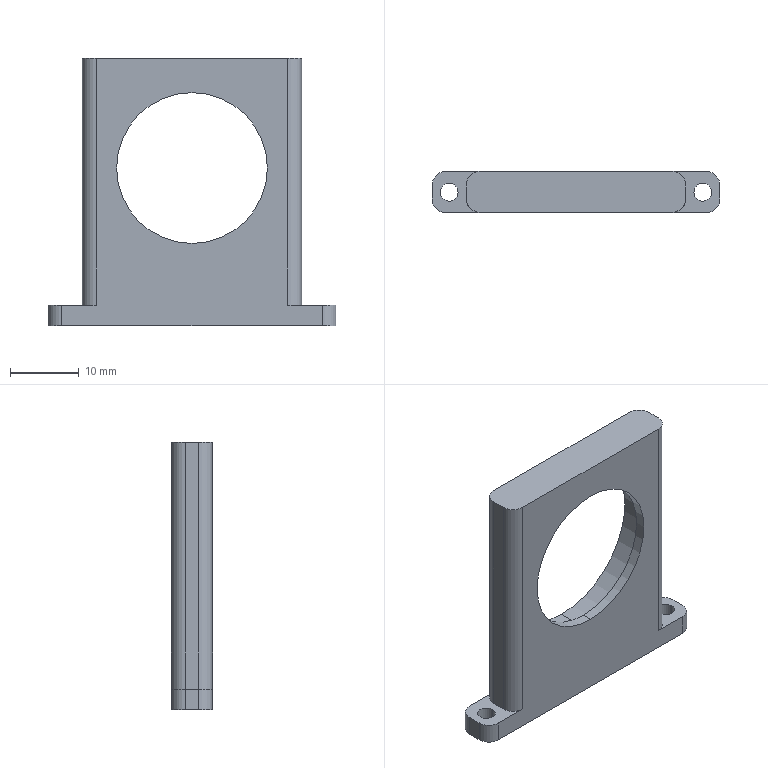Part | NX | 1 solid | 31 faces | box 42 x 6 x 39 mm | volume 4443 mm3 | cylinder 18 | plane 11 | cone 2 | commonest cylinder face diameters 4 x8 2.6 x4 3.3 x2 22 x2 26.2 x2
STEP:
#1=CARTESIAN_POINT('',(1.65,0.,4.009));
#2=VERTEX_POINT('',#1);
#3=CARTESIAN_POINT('',(-1.65,0.,4.009));
#4=VERTEX_POINT('',#3);
#5=CARTESIAN_POINT('',(0.,0.,4.009));
#6=DIRECTION('',(0.,0.,-1.));
#7=DIRECTION('',(-1.,0.,0.));
#8=AXIS2_PLACEMENT_3D('',#5,#6,#7);
#9=CIRCLE('',#8,1.65);
#10=EDGE_CURVE('',#2,#4,#9,.T.);
#11=ORIENTED_EDGE('',*,*,#10,.F.);
#12=CARTESIAN_POINT('',(1.65,0.,-3.));
#13=VERTEX_POINT('',#12);
#14=CARTESIAN_POINT('',(1.65,0.,-3.));
#15=DIRECTION('',(0.,0.,-1.));
#16=VECTOR('',#15,1000.);
#17=LINE('',#14,#16);
#18=EDGE_CURVE('',#2,#13,#17,.T.);
#19=ORIENTED_EDGE('',*,*,#18,.T.);
#20=CARTESIAN_POINT('',(-1.65,0.,-3.));
#21=VERTEX_POINT('',#20);
#22=CARTESIAN_POINT('',(0.,0.,-3.));
#23=DIRECTION('',(0.,0.,-1.));
#24=DIRECTION('',(-1.,0.,0.));
#25=AXIS2_PLACEMENT_3D('',#22,#23,#24);
#26=CIRCLE('',#25,1.65);
#27=EDGE_CURVE('',#13,#21,#26,.T.);
#28=ORIENTED_EDGE('',*,*,#27,.T.);
#29=CARTESIAN_POINT('',(-1.65,0.,-3.));
#30=DIRECTION('',(0.,0.,-1.));
#31=VECTOR('',#30,1000.);
#32=LINE('',#29,#31);
#33=EDGE_CURVE('',#4,#21,#32,.T.);
#34=ORIENTED_EDGE('',*,*,#33,.F.);
#35=EDGE_LOOP('',(#11,#19,#28,#34));
#36=FACE_BOUND('',#35,.T.);
#37=CARTESIAN_POINT('',(0.,0.,-3.));
#38=DIRECTION('',(0.,0.,-1.));
#39=DIRECTION('',(1.,0.,0.));
#40=AXIS2_PLACEMENT_3D('',#37,#38,#39);
#41=CYLINDRICAL_SURFACE('',#40,1.65);
#42=ADVANCED_FACE('',(#36),#41,.F.);
#43=CARTESIAN_POINT('',(0.,0.,5.));
#44=VERTEX_POINT('',#43);
#45=CARTESIAN_POINT('',(-1.65,0.,4.009));
#46=DIRECTION('',(-0.8572,0.,-0.515));
#47=VECTOR('',#46,1000.);
#48=LINE('',#45,#47);
#49=EDGE_CURVE('',#44,#4,#48,.T.);
#50=ORIENTED_EDGE('',*,*,#49,.F.);
#51=CARTESIAN_POINT('',(1.65,0.,4.009));
#52=DIRECTION('',(0.8572,0.,-0.515));
#53=VECTOR('',#52,1000.);
#54=LINE('',#51,#53);
#55=EDGE_CURVE('',#44,#2,#54,.T.);
#56=ORIENTED_EDGE('',*,*,#55,.T.);
#57=ORIENTED_EDGE('',*,*,#10,.T.);
#58=EDGE_LOOP('',(#50,#56,#57));
#59=FACE_BOUND('',#58,.T.);
#60=CARTESIAN_POINT('',(0.,0.,4.009));
#61=DIRECTION('',(0.,0.,-1.));
#62=DIRECTION('',(1.,0.,0.));
#63=AXIS2_PLACEMENT_3D('',#60,#61,#62);
#64=CONICAL_SURFACE('',#63,1.65,1.03);
#65=ADVANCED_FACE('',(#59),#64,.F.);
#66=CARTESIAN_POINT('',(19.8,0.,0.));
#67=VERTEX_POINT('',#66);
#68=CARTESIAN_POINT('',(17.2,0.,0.));
#69=VERTEX_POINT('',#68);
#70=CARTESIAN_POINT('',(18.5,0.,0.));
#71=DIRECTION('',(0.,0.,-1.));
#72=DIRECTION('',(-1.,0.,0.));
#73=AXIS2_PLACEMENT_3D('',#70,#71,#72);
#74=CIRCLE('',#73,1.3);
#75=EDGE_CURVE('',#67,#69,#74,.T.);
#76=ORIENTED_EDGE('',*,*,#75,.F.);
#77=CARTESIAN_POINT('',(19.8,0.,-3.));
#78=VERTEX_POINT('',#77);
#79=CARTESIAN_POINT('',(19.8,0.,36.));
#80=DIRECTION('',(0.,0.,-1.));
#81=VECTOR('',#80,1000.);
#82=LINE('',#79,#81);
#83=EDGE_CURVE('',#67,#78,#82,.T.);
#84=ORIENTED_EDGE('',*,*,#83,.T.);
#85=CARTESIAN_POINT('',(17.2,0.,-3.));
#86=VERTEX_POINT('',#85);
#87=CARTESIAN_POINT('',(18.5,0.,-3.));
#88=DIRECTION('',(0.,0.,-1.));
#89=DIRECTION('',(-1.,0.,0.));
#90=AXIS2_PLACEMENT_3D('',#87,#88,#89);
#91=CIRCLE('',#90,1.3);
#92=EDGE_CURVE('',#78,#86,#91,.T.);
#93=ORIENTED_EDGE('',*,*,#92,.T.);
#94=CARTESIAN_POINT('',(17.2,0.,36.));
#95=DIRECTION('',(0.,0.,-1.));
#96=VECTOR('',#95,1000.);
#97=LINE('',#94,#96);
#98=EDGE_CURVE('',#69,#86,#97,.T.);
#99=ORIENTED_EDGE('',*,*,#98,.F.);
#100=EDGE_LOOP('',(#76,#84,#93,#99));
#101=FACE_BOUND('',#100,.T.);
#102=CARTESIAN_POINT('',(18.5,0.,36.));
#103=DIRECTION('',(0.,0.,-1.));
#104=DIRECTION('',(1.,0.,0.));
#105=AXIS2_PLACEMENT_3D('',#102,#103,#104);
#106=CYLINDRICAL_SURFACE('',#105,1.3);
#107=ADVANCED_FACE('',(#101),#106,.F.);
#108=CARTESIAN_POINT('',(-17.2,0.,0.));
#109=VERTEX_POINT('',#108);
#110=CARTESIAN_POINT('',(-19.8,0.,0.));
#111=VERTEX_POINT('',#110);
#112=CARTESIAN_POINT('',(-18.5,0.,0.));
#113=DIRECTION('',(0.,0.,-1.));
#114=DIRECTION('',(-1.,0.,0.));
#115=AXIS2_PLACEMENT_3D('',#112,#113,#114);
#116=CIRCLE('',#115,1.3);
#117=EDGE_CURVE('',#109,#111,#116,.T.);
#118=ORIENTED_EDGE('',*,*,#117,.F.);
#119=CARTESIAN_POINT('',(-17.2,0.,-3.));
#120=VERTEX_POINT('',#119);
#121=CARTESIAN_POINT('',(-17.2,0.,36.));
#122=DIRECTION('',(0.,0.,-1.));
#123=VECTOR('',#122,1000.);
#124=LINE('',#121,#123);
#125=EDGE_CURVE('',#109,#120,#124,.T.);
#126=ORIENTED_EDGE('',*,*,#125,.T.);
#127=CARTESIAN_POINT('',(-19.8,0.,-3.));
#128=VERTEX_POINT('',#127);
#129=CARTESIAN_POINT('',(-18.5,0.,-3.));
#130=DIRECTION('',(0.,0.,-1.));
#131=DIRECTION('',(-1.,0.,0.));
#132=AXIS2_PLACEMENT_3D('',#129,#130,#131);
#133=CIRCLE('',#132,1.3);
#134=EDGE_CURVE('',#120,#128,#133,.T.);
#135=ORIENTED_EDGE('',*,*,#134,.T.);
#136=CARTESIAN_POINT('',(-19.8,0.,36.));
#137=DIRECTION('',(0.,0.,-1.));
#138=VECTOR('',#137,1000.);
#139=LINE('',#136,#138);
#140=EDGE_CURVE('',#111,#128,#139,.T.);
#141=ORIENTED_EDGE('',*,*,#140,.F.);
#142=EDGE_LOOP('',(#118,#126,#135,#141));
#143=FACE_BOUND('',#142,.T.);
#144=CARTESIAN_POINT('',(-18.5,0.,36.));
#145=DIRECTION('',(0.,0.,-1.));
#146=DIRECTION('',(1.,0.,0.));
#147=AXIS2_PLACEMENT_3D('',#144,#145,#146);
#148=CYLINDRICAL_SURFACE('',#147,1.3);
#149=ADVANCED_FACE('',(#143),#148,.F.);
#150=CARTESIAN_POINT('',(0.,-1.5,6.9));
#151=VERTEX_POINT('',#150);
#152=CARTESIAN_POINT('',(0.,-1.5,33.1));
#153=VERTEX_POINT('',#152);
#154=CARTESIAN_POINT('',(0.,-1.5,20.));
#155=DIRECTION('',(0.,1.,0.));
#156=DIRECTION('',(0.,0.,1.));
#157=AXIS2_PLACEMENT_3D('',#154,#155,#156);
#158=CIRCLE('',#157,13.1);
#159=EDGE_CURVE('',#151,#153,#158,.T.);
#160=ORIENTED_EDGE('',*,*,#159,.F.);
#161=CARTESIAN_POINT('',(0.,3.,6.9));
#162=VERTEX_POINT('',#161);
#163=CARTESIAN_POINT('',(0.,-1.5,6.9));
#164=DIRECTION('',(0.,1.,0.));
#165=VECTOR('',#164,1000.);
#166=LINE('',#163,#165);
#167=EDGE_CURVE('',#151,#162,#166,.T.);
#168=ORIENTED_EDGE('',*,*,#167,.T.);
#169=CARTESIAN_POINT('',(0.,3.,33.1));
#170=VERTEX_POINT('',#169);
#171=CARTESIAN_POINT('',(0.,3.,20.));
#172=DIRECTION('',(0.,1.,0.));
#173=DIRECTION('',(0.,0.,1.));
#174=AXIS2_PLACEMENT_3D('',#171,#172,#173);
#175=CIRCLE('',#174,13.1);
#176=EDGE_CURVE('',#162,#170,#175,.T.);
#177=ORIENTED_EDGE('',*,*,#176,.T.);
#178=CARTESIAN_POINT('',(0.,-1.5,33.1));
#179=DIRECTION('',(0.,1.,0.));
#180=VECTOR('',#179,1000.);
#181=LINE('',#178,#180);
#182=EDGE_CURVE('',#153,#170,#181,.T.);
#183=ORIENTED_EDGE('',*,*,#182,.F.);
#184=EDGE_LOOP('',(#160,#168,#177,#183));
#185=FACE_BOUND('',#184,.T.);
#186=CARTESIAN_POINT('',(0.,-1.5,20.));
#187=DIRECTION('',(0.,1.,0.));
#188=DIRECTION('',(0.,0.,-1.));
#189=AXIS2_PLACEMENT_3D('',#186,#187,#188);
#190=CYLINDRICAL_SURFACE('',#189,13.1);
#191=ADVANCED_FACE('',(#185),#190,.F.);
#192=CARTESIAN_POINT('',(0.,-1.5,31.));
#193=VERTEX_POINT('',#192);
#194=CARTESIAN_POINT('',(0.,-1.5,9.));
#195=VERTEX_POINT('',#194);
#196=CARTESIAN_POINT('',(0.,-1.5,20.));
#197=DIRECTION('',(0.,-1.,0.));
#198=DIRECTION('',(0.,0.,1.));
#199=AXIS2_PLACEMENT_3D('',#196,#197,#198);
#200=CIRCLE('',#199,11.);
#201=EDGE_CURVE('',#193,#195,#200,.T.);
#202=ORIENTED_EDGE('',*,*,#201,.F.);
#203=CARTESIAN_POINT('',(0.,-3.,31.));
#204=VERTEX_POINT('',#203);
#205=CARTESIAN_POINT('',(0.,3.,31.));
#206=DIRECTION('',(0.,-1.,0.));
#207=VECTOR('',#206,1000.);
#208=LINE('',#205,#207);
#209=EDGE_CURVE('',#193,#204,#208,.T.);
#210=ORIENTED_EDGE('',*,*,#209,.T.);
#211=CARTESIAN_POINT('',(0.,-3.,9.));
#212=VERTEX_POINT('',#211);
#213=CARTESIAN_POINT('',(0.,-3.,20.));
#214=DIRECTION('',(0.,-1.,0.));
#215=DIRECTION('',(0.,0.,-1.));
#216=AXIS2_PLACEMENT_3D('',#213,#214,#215);
#217=CIRCLE('',#216,11.);
#218=EDGE_CURVE('',#204,#212,#217,.T.);
#219=ORIENTED_EDGE('',*,*,#218,.T.);
#220=CARTESIAN_POINT('',(0.,3.,9.));
#221=DIRECTION('',(0.,-1.,0.));
#222=VECTOR('',#221,1000.);
#223=LINE('',#220,#222);
#224=EDGE_CURVE('',#195,#212,#223,.T.);
#225=ORIENTED_EDGE('',*,*,#224,.F.);
#226=EDGE_LOOP('',(#202,#210,#219,#225));
#227=FACE_BOUND('',#226,.T.);
#228=CARTESIAN_POINT('',(0.,3.,20.));
#229=DIRECTION('',(0.,-1.,0.));
#230=DIRECTION('',(0.,0.,1.));
#231=AXIS2_PLACEMENT_3D('',#228,#229,#230);
#232=CYLINDRICAL_SURFACE('',#231,11.);
#233=ADVANCED_FACE('',(#227),#232,.F.);
#234=ORIENTED_EDGE('',*,*,#209,.F.);
#235=CARTESIAN_POINT('',(0.,-1.5,20.));
#236=DIRECTION('',(0.,-1.,0.));
#237=DIRECTION('',(0.,0.,1.));
#238=AXIS2_PLACEMENT_3D('',#235,#236,#237);
#239=CIRCLE('',#238,11.);
#240=EDGE_CURVE('',#195,#193,#239,.T.);
#241=ORIENTED_EDGE('',*,*,#240,.F.);
#242=ORIENTED_EDGE('',*,*,#224,.T.);
#243=CARTESIAN_POINT('',(0.,-3.,20.));
#244=DIRECTION('',(0.,-1.,0.));
#245=DIRECTION('',(0.,0.,-1.));
#246=AXIS2_PLACEMENT_3D('',#243,#244,#245);
#247=CIRCLE('',#246,11.);
#248=EDGE_CURVE('',#212,#204,#247,.T.);
#249=ORIENTED_EDGE('',*,*,#248,.T.);
#250=EDGE_LOOP('',(#234,#241,#242,#249));
#251=FACE_BOUND('',#250,.T.);
#252=CARTESIAN_POINT('',(0.,3.,20.));
#253=DIRECTION('',(0.,-1.,0.));
#254=DIRECTION('',(0.,0.,1.));
#255=AXIS2_PLACEMENT_3D('',#252,#253,#254);
#256=CYLINDRICAL_SURFACE('',#255,11.);
#257=ADVANCED_FACE('',(#251),#256,.F.);
#258=CARTESIAN_POINT('',(16.,-1.,36.));
#259=VERTEX_POINT('',#258);
#260=CARTESIAN_POINT('',(16.,1.,36.));
#261=VERTEX_POINT('',#260);
#262=CARTESIAN_POINT('',(16.,-3.,36.));
#263=DIRECTION('',(0.,1.,0.));
#264=VECTOR('',#263,1000.);
#265=LINE('',#262,#264);
#266=EDGE_CURVE('',#259,#261,#265,.T.);
#267=ORIENTED_EDGE('',*,*,#266,.F.);
#268=CARTESIAN_POINT('',(16.,-1.,0.));
#269=VERTEX_POINT('',#268);
#270=CARTESIAN_POINT('',(16.,-1.,36.));
#271=DIRECTION('',(0.,0.,-1.));
#272=VECTOR('',#271,1000.);
#273=LINE('',#270,#272);
#274=EDGE_CURVE('',#259,#269,#273,.T.);
#275=ORIENTED_EDGE('',*,*,#274,.T.);
#276=CARTESIAN_POINT('',(16.,1.,0.));
#277=VERTEX_POINT('',#276);
#278=CARTESIAN_POINT('',(16.,-3.,0.));
#279=DIRECTION('',(0.,1.,0.));
#280=VECTOR('',#279,1000.);
#281=LINE('',#278,#280);
#282=EDGE_CURVE('',#269,#277,#281,.T.);
#283=ORIENTED_EDGE('',*,*,#282,.T.);
#284=CARTESIAN_POINT('',(16.,1.,36.));
#285=DIRECTION('',(0.,0.,1.));
#286=VECTOR('',#285,1000.);
#287=LINE('',#284,#286);
#288=EDGE_CURVE('',#277,#261,#287,.T.);
#289=ORIENTED_EDGE('',*,*,#288,.T.);
#290=EDGE_LOOP('',(#267,#275,#283,#289));
#291=FACE_BOUND('',#290,.T.);
#292=CARTESIAN_POINT('',(16.,-3.,36.));
#293=DIRECTION('',(-1.,0.,0.));
#294=DIRECTION('',(0.,0.,-1.));
#295=AXIS2_PLACEMENT_3D('',#292,#293,#294);
#296=PLANE('',#295);
#297=ADVANCED_FACE('',(#291),#296,.F.);
#298=CARTESIAN_POINT('',(0.,3.,20.));
#299=DIRECTION('',(0.,1.,0.));
#300=DIRECTION('',(0.,0.,1.));
#301=AXIS2_PLACEMENT_3D('',#298,#299,#300);
#302=CIRCLE('',#301,13.1);
#303=EDGE_CURVE('',#170,#162,#302,.T.);
#304=ORIENTED_EDGE('',*,*,#303,.F.);
#305=ORIENTED_EDGE('',*,*,#176,.F.);
#306=EDGE_LOOP('',(#304,#305));
#307=FACE_BOUND('',#306,.T.);
#308=CARTESIAN_POINT('',(14.,3.,0.));
#309=VERTEX_POINT('',#308);
#310=CARTESIAN_POINT('',(19.,3.,0.));
#311=VERTEX_POINT('',#310);
#312=CARTESIAN_POINT('',(-21.,3.,0.));
#313=DIRECTION('',(1.,0.,0.));
#314=VECTOR('',#313,1000.);
#315=LINE('',#312,#314);
#316=EDGE_CURVE('',#309,#311,#315,.T.);
#317=ORIENTED_EDGE('',*,*,#316,.T.);
#318=CARTESIAN_POINT('',(19.,3.,-3.));
#319=VERTEX_POINT('',#318);
#320=CARTESIAN_POINT('',(19.,3.,-3.));
#321=DIRECTION('',(0.,0.,-1.));
#322=VECTOR('',#321,1000.);
#323=LINE('',#320,#322);
#324=EDGE_CURVE('',#311,#319,#323,.T.);
#325=ORIENTED_EDGE('',*,*,#324,.T.);
#326=CARTESIAN_POINT('',(-19.,3.,-3.));
#327=VERTEX_POINT('',#326);
#328=CARTESIAN_POINT('',(-21.,3.,-3.));
#329=DIRECTION('',(1.,0.,0.));
#330=VECTOR('',#329,1000.);
#331=LINE('',#328,#330);
#332=EDGE_CURVE('',#327,#319,#331,.T.);
#333=ORIENTED_EDGE('',*,*,#332,.F.);
#334=CARTESIAN_POINT('',(-19.,3.,0.));
#335=VERTEX_POINT('',#334);
#336=CARTESIAN_POINT('',(-19.,3.,36.));
#337=DIRECTION('',(0.,0.,1.));
#338=VECTOR('',#337,1000.);
#339=LINE('',#336,#338);
#340=EDGE_CURVE('',#327,#335,#339,.T.);
#341=ORIENTED_EDGE('',*,*,#340,.T.);
#342=CARTESIAN_POINT('',(-14.,3.,0.));
#343=VERTEX_POINT('',#342);
#344=CARTESIAN_POINT('',(-21.,3.,0.));
#345=DIRECTION('',(1.,0.,0.));
#346=VECTOR('',#345,1000.);
#347=LINE('',#344,#346);
#348=EDGE_CURVE('',#335,#343,#347,.T.);
#349=ORIENTED_EDGE('',*,*,#348,.T.);
#350=CARTESIAN_POINT('',(-14.,3.,36.));
#351=VERTEX_POINT('',#350);
#352=CARTESIAN_POINT('',(-14.,3.,36.));
#353=DIRECTION('',(0.,0.,1.));
#354=VECTOR('',#353,1000.);
#355=LINE('',#352,#354);
#356=EDGE_CURVE('',#343,#351,#355,.T.);
#357=ORIENTED_EDGE('',*,*,#356,.T.);
#358=CARTESIAN_POINT('',(14.,3.,36.));
#359=VERTEX_POINT('',#358);
#360=CARTESIAN_POINT('',(-16.,3.,36.));
#361=DIRECTION('',(-1.,0.,0.));
#362=VECTOR('',#361,1000.);
#363=LINE('',#360,#362);
#364=EDGE_CURVE('',#359,#351,#363,.T.);
#365=ORIENTED_EDGE('',*,*,#364,.F.);
#366=CARTESIAN_POINT('',(14.,3.,36.));
#367=DIRECTION('',(0.,0.,-1.));
#368=VECTOR('',#367,1000.);
#369=LINE('',#366,#368);
#370=EDGE_CURVE('',#359,#309,#369,.T.);
#371=ORIENTED_EDGE('',*,*,#370,.T.);
#372=EDGE_LOOP('',(#317,#325,#333,#341,#349,#357,#365,#371));
#373=FACE_BOUND('',#372,.T.);
#374=CARTESIAN_POINT('',(-16.,3.,36.));
#375=DIRECTION('',(0.,-1.,0.));
#376=DIRECTION('',(0.,0.,1.));
#377=AXIS2_PLACEMENT_3D('',#374,#375,#376);
#378=PLANE('',#377);
#379=ADVANCED_FACE('',(#307,#373),#378,.F.);
#380=CARTESIAN_POINT('',(-16.,1.,36.));
#381=VERTEX_POINT('',#380);
#382=CARTESIAN_POINT('',(-16.,-1.,36.));
#383=VERTEX_POINT('',#382);
#384=CARTESIAN_POINT('',(-16.,-3.,36.));
#385=DIRECTION('',(0.,-1.,0.));
#386=VECTOR('',#385,1000.);
#387=LINE('',#384,#386);
#388=EDGE_CURVE('',#381,#383,#387,.T.);
#389=ORIENTED_EDGE('',*,*,#388,.F.);
#390=CARTESIAN_POINT('',(-16.,1.,0.));
#391=VERTEX_POINT('',#390);
#392=CARTESIAN_POINT('',(-16.,1.,36.));
#393=DIRECTION('',(0.,0.,-1.));
#394=VECTOR('',#393,1000.);
#395=LINE('',#392,#394);
#396=EDGE_CURVE('',#381,#391,#395,.T.);
#397=ORIENTED_EDGE('',*,*,#396,.T.);
#398=CARTESIAN_POINT('',(-16.,-1.,0.));
#399=VERTEX_POINT('',#398);
#400=CARTESIAN_POINT('',(-16.,-3.,0.));
#401=DIRECTION('',(0.,-1.,0.));
#402=VECTOR('',#401,1000.);
#403=LINE('',#400,#402);
#404=EDGE_CURVE('',#391,#399,#403,.T.);
#405=ORIENTED_EDGE('',*,*,#404,.T.);
#406=CARTESIAN_POINT('',(-16.,-1.,36.));
#407=DIRECTION('',(0.,0.,1.));
#408=VECTOR('',#407,1000.);
#409=LINE('',#406,#408);
#410=EDGE_CURVE('',#399,#383,#409,.T.);
#411=ORIENTED_EDGE('',*,*,#410,.T.);
#412=EDGE_LOOP('',(#389,#397,#405,#411));
#413=FACE_BOUND('',#412,.T.);
#414=CARTESIAN_POINT('',(-16.,-3.,36.));
#415=DIRECTION('',(1.,0.,0.));
#416=DIRECTION('',(0.,0.,1.));
#417=AXIS2_PLACEMENT_3D('',#414,#415,#416);
#418=PLANE('',#417);
#419=ADVANCED_FACE('',(#413),#418,.F.);
#420=ORIENTED_EDGE('',*,*,#248,.F.);
#421=ORIENTED_EDGE('',*,*,#218,.F.);
#422=EDGE_LOOP('',(#420,#421));
#423=FACE_BOUND('',#422,.T.);
#424=CARTESIAN_POINT('',(-19.,-3.,-3.));
#425=VERTEX_POINT('',#424);
#426=CARTESIAN_POINT('',(19.,-3.,-3.));
#427=VERTEX_POINT('',#426);
#428=CARTESIAN_POINT('',(-21.,-3.,-3.));
#429=DIRECTION('',(1.,0.,0.));
#430=VECTOR('',#429,1000.);
#431=LINE('',#428,#430);
#432=EDGE_CURVE('',#425,#427,#431,.T.);
#433=ORIENTED_EDGE('',*,*,#432,.T.);
#434=CARTESIAN_POINT('',(19.,-3.,0.));
#435=VERTEX_POINT('',#434);
#436=CARTESIAN_POINT('',(19.,-3.,0.));
#437=DIRECTION('',(0.,0.,1.));
#438=VECTOR('',#437,1000.);
#439=LINE('',#436,#438);
#440=EDGE_CURVE('',#427,#435,#439,.T.);
#441=ORIENTED_EDGE('',*,*,#440,.T.);
#442=CARTESIAN_POINT('',(14.,-3.,0.));
#443=VERTEX_POINT('',#442);
#444=CARTESIAN_POINT('',(-21.,-3.,0.));
#445=DIRECTION('',(1.,0.,0.));
#446=VECTOR('',#445,1000.);
#447=LINE('',#444,#446);
#448=EDGE_CURVE('',#443,#435,#447,.T.);
#449=ORIENTED_EDGE('',*,*,#448,.F.);
#450=CARTESIAN_POINT('',(14.,-3.,36.));
#451=VERTEX_POINT('',#450);
#452=CARTESIAN_POINT('',(14.,-3.,36.));
#453=DIRECTION('',(0.,0.,1.));
#454=VECTOR('',#453,1000.);
#455=LINE('',#452,#454);
#456=EDGE_CURVE('',#443,#451,#455,.T.);
#457=ORIENTED_EDGE('',*,*,#456,.T.);
#458=CARTESIAN_POINT('',(-14.,-3.,36.));
#459=VERTEX_POINT('',#458);
#460=CARTESIAN_POINT('',(-16.,-3.,36.));
#461=DIRECTION('',(1.,0.,0.));
#462=VECTOR('',#461,1000.);
#463=LINE('',#460,#462);
#464=EDGE_CURVE('',#459,#451,#463,.T.);
#465=ORIENTED_EDGE('',*,*,#464,.F.);
#466=CARTESIAN_POINT('',(-14.,-3.,0.));
#467=VERTEX_POINT('',#466);
#468=CARTESIAN_POINT('',(-14.,-3.,36.));
#469=DIRECTION('',(0.,0.,-1.));
#470=VECTOR('',#469,1000.);
#471=LINE('',#468,#470);
#472=EDGE_CURVE('',#459,#467,#471,.T.);
#473=ORIENTED_EDGE('',*,*,#472,.T.);
#474=CARTESIAN_POINT('',(-19.,-3.,0.));
#475=VERTEX_POINT('',#474);
#476=CARTESIAN_POINT('',(-21.,-3.,0.));
#477=DIRECTION('',(1.,0.,0.));
#478=VECTOR('',#477,1000.);
#479=LINE('',#476,#478);
#480=EDGE_CURVE('',#475,#467,#479,.T.);
#481=ORIENTED_EDGE('',*,*,#480,.F.);
#482=CARTESIAN_POINT('',(-19.,-3.,36.));
#483=DIRECTION('',(0.,0.,-1.));
#484=VECTOR('',#483,1000.);
#485=LINE('',#482,#484);
#486=EDGE_CURVE('',#475,#425,#485,.T.);
#487=ORIENTED_EDGE('',*,*,#486,.T.);
#488=EDGE_LOOP('',(#433,#441,#449,#457,#465,#473,#481,#487));
#489=FACE_BOUND('',#488,.T.);
#490=CARTESIAN_POINT('',(-16.,-3.,36.));
#491=DIRECTION('',(0.,1.,0.));
#492=DIRECTION('',(0.,0.,-1.));
#493=AXIS2_PLACEMENT_3D('',#490,#491,#492);
#494=PLANE('',#493);
#495=ADVANCED_FACE('',(#423,#489),#494,.F.);
#496=ORIENTED_EDGE('',*,*,#464,.T.);
#497=CARTESIAN_POINT('',(14.,-1.,36.));
#498=DIRECTION('',(0.,0.,1.));
#499=DIRECTION('',(-1.,0.,0.));
#500=AXIS2_PLACEMENT_3D('',#497,#498,#499);
#501=CIRCLE('',#500,2.);
#502=EDGE_CURVE('',#451,#259,#501,.T.);
#503=ORIENTED_EDGE('',*,*,#502,.T.);
#504=ORIENTED_EDGE('',*,*,#266,.T.);
#505=CARTESIAN_POINT('',(14.,1.,36.));
#506=DIRECTION('',(0.,0.,1.));
#507=DIRECTION('',(-1.,0.,0.));
#508=AXIS2_PLACEMENT_3D('',#505,#506,#507);
#509=CIRCLE('',#508,2.);
#510=EDGE_CURVE('',#261,#359,#509,.T.);
#511=ORIENTED_EDGE('',*,*,#510,.T.);
#512=ORIENTED_EDGE('',*,*,#364,.T.);
#513=CARTESIAN_POINT('',(-14.,1.,36.));
#514=DIRECTION('',(0.,0.,1.));
#515=DIRECTION('',(-1.,0.,0.));
#516=AXIS2_PLACEMENT_3D('',#513,#514,#515);
#517=CIRCLE('',#516,2.);
#518=EDGE_CURVE('',#351,#381,#517,.T.);
#519=ORIENTED_EDGE('',*,*,#518,.T.);
#520=ORIENTED_EDGE('',*,*,#388,.T.);
#521=CARTESIAN_POINT('',(-14.,-1.,36.));
#522=DIRECTION('',(0.,0.,1.));
#523=DIRECTION('',(-1.,0.,0.));
#524=AXIS2_PLACEMENT_3D('',#521,#522,#523);
#525=CIRCLE('',#524,2.);
#526=EDGE_CURVE('',#383,#459,#525,.T.);
#527=ORIENTED_EDGE('',*,*,#526,.T.);
#528=EDGE_LOOP('',(#496,#503,#504,#511,#512,#519,#520,#527));
#529=FACE_BOUND('',#528,.T.);
#530=CARTESIAN_POINT('',(0.,0.,36.));
#531=DIRECTION('',(0.,0.,-1.));
#532=DIRECTION('',(1.,0.,0.));
#533=AXIS2_PLACEMENT_3D('',#530,#531,#532);
#534=PLANE('',#533);
#535=ADVANCED_FACE('',(#529),#534,.F.);
#536=CARTESIAN_POINT('',(18.5,0.,0.));
#537=DIRECTION('',(0.,0.,-1.));
#538=DIRECTION('',(-1.,0.,0.));
#539=AXIS2_PLACEMENT_3D('',#536,#537,#538);
#540=CIRCLE('',#539,1.3);
#541=EDGE_CURVE('',#69,#67,#540,.T.);
#542=ORIENTED_EDGE('',*,*,#541,.T.);
#543=ORIENTED_EDGE('',*,*,#75,.T.);
#544=EDGE_LOOP('',(#542,#543));
#545=FACE_BOUND('',#544,.T.);
#546=ORIENTED_EDGE('',*,*,#448,.T.);
#547=CARTESIAN_POINT('',(21.,-1.,0.));
#548=VERTEX_POINT('',#547);
#549=CARTESIAN_POINT('',(19.,-1.,0.));
#550=DIRECTION('',(0.,0.,1.));
#551=DIRECTION('',(-1.,0.,0.));
#552=AXIS2_PLACEMENT_3D('',#549,#550,#551);
#553=CIRCLE('',#552,2.);
#554=EDGE_CURVE('',#435,#548,#553,.T.);
#555=ORIENTED_EDGE('',*,*,#554,.T.);
#556=CARTESIAN_POINT('',(21.,1.,0.));
#557=VERTEX_POINT('',#556);
#558=CARTESIAN_POINT('',(21.,-3.,0.));
#559=DIRECTION('',(0.,1.,0.));
#560=VECTOR('',#559,1000.);
#561=LINE('',#558,#560);
#562=EDGE_CURVE('',#548,#557,#561,.T.);
#563=ORIENTED_EDGE('',*,*,#562,.T.);
#564=CARTESIAN_POINT('',(19.,1.,0.));
#565=DIRECTION('',(0.,0.,1.));
#566=DIRECTION('',(-1.,0.,0.));
#567=AXIS2_PLACEMENT_3D('',#564,#565,#566);
#568=CIRCLE('',#567,2.);
#569=EDGE_CURVE('',#557,#311,#568,.T.);
#570=ORIENTED_EDGE('',*,*,#569,.T.);
#571=ORIENTED_EDGE('',*,*,#316,.F.);
#572=CARTESIAN_POINT('',(14.,1.,0.));
#573=DIRECTION('',(0.,0.,-1.));
#574=DIRECTION('',(-1.,0.,0.));
#575=AXIS2_PLACEMENT_3D('',#572,#573,#574);
#576=CIRCLE('',#575,2.);
#577=EDGE_CURVE('',#309,#277,#576,.T.);
#578=ORIENTED_EDGE('',*,*,#577,.T.);
#579=ORIENTED_EDGE('',*,*,#282,.F.);
#580=CARTESIAN_POINT('',(14.,-1.,0.));
#581=DIRECTION('',(0.,0.,-1.));
#582=DIRECTION('',(-1.,0.,0.));
#583=AXIS2_PLACEMENT_3D('',#580,#581,#582);
#584=CIRCLE('',#583,2.);
#585=EDGE_CURVE('',#269,#443,#584,.T.);
#586=ORIENTED_EDGE('',*,*,#585,.T.);
#587=EDGE_LOOP('',(#546,#555,#563,#570,#571,#578,#579,#586));
#588=FACE_BOUND('',#587,.T.);
#589=CARTESIAN_POINT('',(0.,0.,0.));
#590=DIRECTION('',(0.,0.,-1.));
#591=DIRECTION('',(1.,0.,0.));
#592=AXIS2_PLACEMENT_3D('',#589,#590,#591);
#593=PLANE('',#592);
#594=ADVANCED_FACE('',(#545,#588),#593,.F.);
#595=CARTESIAN_POINT('',(-21.,-1.,0.));
#596=VERTEX_POINT('',#595);
#597=CARTESIAN_POINT('',(-21.,1.,0.));
#598=VERTEX_POINT('',#597);
#599=CARTESIAN_POINT('',(-21.,-3.,0.));
#600=DIRECTION('',(0.,1.,0.));
#601=VECTOR('',#600,1000.);
#602=LINE('',#599,#601);
#603=EDGE_CURVE('',#596,#598,#602,.T.);
#604=ORIENTED_EDGE('',*,*,#603,.T.);
#605=CARTESIAN_POINT('',(-21.,1.,-3.));
#606=VERTEX_POINT('',#605);
#607=CARTESIAN_POINT('',(-21.,1.,-3.));
#608=DIRECTION('',(0.,0.,-1.));
#609=VECTOR('',#608,1000.);
#610=LINE('',#607,#609);
#611=EDGE_CURVE('',#598,#606,#610,.T.);
#612=ORIENTED_EDGE('',*,*,#611,.T.);
#613=CARTESIAN_POINT('',(-21.,-1.,-3.));
#614=VERTEX_POINT('',#613);
#615=CARTESIAN_POINT('',(-21.,-3.,-3.));
#616=DIRECTION('',(0.,1.,0.));
#617=VECTOR('',#616,1000.);
#618=LINE('',#615,#617);
#619=EDGE_CURVE('',#614,#606,#618,.T.);
#620=ORIENTED_EDGE('',*,*,#619,.F.);
#621=CARTESIAN_POINT('',(-21.,-1.,-3.));
#622=DIRECTION('',(0.,0.,1.));
#623=VECTOR('',#622,1000.);
#624=LINE('',#621,#623);
#625=EDGE_CURVE('',#614,#596,#624,.T.);
#626=ORIENTED_EDGE('',*,*,#625,.T.);
#627=EDGE_LOOP('',(#604,#612,#620,#626));
#628=FACE_BOUND('',#627,.T.);
#629=CARTESIAN_POINT('',(-21.,-3.,-3.));
#630=DIRECTION('',(1.,0.,0.));
#631=DIRECTION('',(0.,0.,1.));
#632=AXIS2_PLACEMENT_3D('',#629,#630,#631);
#633=PLANE('',#632);
#634=ADVANCED_FACE('',(#628),#633,.F.);
#635=ORIENTED_EDGE('',*,*,#562,.F.);
#636=CARTESIAN_POINT('',(21.,-1.,-3.));
#637=VERTEX_POINT('',#636);
#638=CARTESIAN_POINT('',(21.,-1.,-3.));
#639=DIRECTION('',(0.,0.,-1.));
#640=VECTOR('',#639,1000.);
#641=LINE('',#638,#640);
#642=EDGE_CURVE('',#548,#637,#641,.T.);
#643=ORIENTED_EDGE('',*,*,#642,.T.);
#644=CARTESIAN_POINT('',(21.,1.,-3.));
#645=VERTEX_POINT('',#644);
#646=CARTESIAN_POINT('',(21.,-3.,-3.));
#647=DIRECTION('',(0.,1.,0.));
#648=VECTOR('',#647,1000.);
#649=LINE('',#646,#648);
#650=EDGE_CURVE('',#637,#645,#649,.T.);
#651=ORIENTED_EDGE('',*,*,#650,.T.);
#652=CARTESIAN_POINT('',(21.,1.,0.));
#653=DIRECTION('',(0.,0.,1.));
#654=VECTOR('',#653,1000.);
#655=LINE('',#652,#654);
#656=EDGE_CURVE('',#645,#557,#655,.T.);
#657=ORIENTED_EDGE('',*,*,#656,.T.);
#658=EDGE_LOOP('',(#635,#643,#651,#657));
#659=FACE_BOUND('',#658,.T.);
#660=CARTESIAN_POINT('',(21.,-3.,-3.));
#661=DIRECTION('',(1.,0.,0.));
#662=DIRECTION('',(0.,0.,1.));
#663=AXIS2_PLACEMENT_3D('',#660,#661,#662);
#664=PLANE('',#663);
#665=ADVANCED_FACE('',(#659),#664,.T.);
#666=CARTESIAN_POINT('',(0.,0.,-3.));
#667=DIRECTION('',(0.,0.,-1.));
#668=DIRECTION('',(-1.,0.,0.));
#669=AXIS2_PLACEMENT_3D('',#666,#667,#668);
#670=CIRCLE('',#669,1.65);
#671=EDGE_CURVE('',#21,#13,#670,.T.);
#672=ORIENTED_EDGE('',*,*,#671,.F.);
#673=ORIENTED_EDGE('',*,*,#27,.F.);
#674=EDGE_LOOP('',(#672,#673));
#675=FACE_BOUND('',#674,.T.);
#676=CARTESIAN_POINT('',(-18.5,0.,-3.));
#677=DIRECTION('',(0.,0.,-1.));
#678=DIRECTION('',(-1.,0.,0.));
#679=AXIS2_PLACEMENT_3D('',#676,#677,#678);
#680=CIRCLE('',#679,1.3);
#681=EDGE_CURVE('',#128,#120,#680,.T.);
#682=ORIENTED_EDGE('',*,*,#681,.F.);
#683=ORIENTED_EDGE('',*,*,#134,.F.);
#684=EDGE_LOOP('',(#682,#683));
#685=FACE_BOUND('',#684,.T.);
#686=CARTESIAN_POINT('',(18.5,0.,-3.));
#687=DIRECTION('',(0.,0.,-1.));
#688=DIRECTION('',(-1.,0.,0.));
#689=AXIS2_PLACEMENT_3D('',#686,#687,#688);
#690=CIRCLE('',#689,1.3);
#691=EDGE_CURVE('',#86,#78,#690,.T.);
#692=ORIENTED_EDGE('',*,*,#691,.F.);
#693=ORIENTED_EDGE('',*,*,#92,.F.);
#694=EDGE_LOOP('',(#692,#693));
#695=FACE_BOUND('',#694,.T.);
#696=ORIENTED_EDGE('',*,*,#650,.F.);
#697=CARTESIAN_POINT('',(19.,-1.,-3.));
#698=DIRECTION('',(0.,0.,-1.));
#699=DIRECTION('',(-1.,0.,0.));
#700=AXIS2_PLACEMENT_3D('',#697,#698,#699);
#701=CIRCLE('',#700,2.);
#702=EDGE_CURVE('',#637,#427,#701,.T.);
#703=ORIENTED_EDGE('',*,*,#702,.T.);
#704=ORIENTED_EDGE('',*,*,#432,.F.);
#705=CARTESIAN_POINT('',(-19.,-1.,-3.));
#706=DIRECTION('',(0.,0.,-1.));
#707=DIRECTION('',(-1.,0.,0.));
#708=AXIS2_PLACEMENT_3D('',#705,#706,#707);
#709=CIRCLE('',#708,2.);
#710=EDGE_CURVE('',#425,#614,#709,.T.);
#711=ORIENTED_EDGE('',*,*,#710,.T.);
#712=ORIENTED_EDGE('',*,*,#619,.T.);
#713=CARTESIAN_POINT('',(-19.,1.,-3.));
#714=DIRECTION('',(0.,0.,-1.));
#715=DIRECTION('',(-1.,0.,0.));
#716=AXIS2_PLACEMENT_3D('',#713,#714,#715);
#717=CIRCLE('',#716,2.);
#718=EDGE_CURVE('',#606,#327,#717,.T.);
#719=ORIENTED_EDGE('',*,*,#718,.T.);
#720=ORIENTED_EDGE('',*,*,#332,.T.);
#721=CARTESIAN_POINT('',(19.,1.,-3.));
#722=DIRECTION('',(0.,0.,-1.));
#723=DIRECTION('',(-1.,0.,0.));
#724=AXIS2_PLACEMENT_3D('',#721,#722,#723);
#725=CIRCLE('',#724,2.);
#726=EDGE_CURVE('',#319,#645,#725,.T.);
#727=ORIENTED_EDGE('',*,*,#726,.T.);
#728=EDGE_LOOP('',(#696,#703,#704,#711,#712,#719,#720,#727));
#729=FACE_BOUND('',#728,.T.);
#730=CARTESIAN_POINT('',(0.,0.,-3.));
#731=DIRECTION('',(0.,0.,-1.));
#732=DIRECTION('',(1.,0.,0.));
#733=AXIS2_PLACEMENT_3D('',#730,#731,#732);
#734=PLANE('',#733);
#735=ADVANCED_FACE('',(#675,#685,#695,#729),#734,.T.);
#736=CARTESIAN_POINT('',(-18.5,0.,0.));
#737=DIRECTION('',(0.,0.,-1.));
#738=DIRECTION('',(-1.,0.,0.));
#739=AXIS2_PLACEMENT_3D('',#736,#737,#738);
#740=CIRCLE('',#739,1.3);
#741=EDGE_CURVE('',#111,#109,#740,.T.);
#742=ORIENTED_EDGE('',*,*,#741,.T.);
#743=ORIENTED_EDGE('',*,*,#117,.T.);
#744=EDGE_LOOP('',(#742,#743));
#745=FACE_BOUND('',#744,.T.);
#746=ORIENTED_EDGE('',*,*,#348,.F.);
#747=CARTESIAN_POINT('',(-19.,1.,0.));
#748=DIRECTION('',(0.,0.,1.));
#749=DIRECTION('',(-1.,0.,0.));
#750=AXIS2_PLACEMENT_3D('',#747,#748,#749);
#751=CIRCLE('',#750,2.);
#752=EDGE_CURVE('',#335,#598,#751,.T.);
#753=ORIENTED_EDGE('',*,*,#752,.T.);
#754=ORIENTED_EDGE('',*,*,#603,.F.);
#755=CARTESIAN_POINT('',(-19.,-1.,0.));
#756=DIRECTION('',(0.,0.,1.));
#757=DIRECTION('',(-1.,0.,0.));
#758=AXIS2_PLACEMENT_3D('',#755,#756,#757);
#759=CIRCLE('',#758,2.);
#760=EDGE_CURVE('',#596,#475,#759,.T.);
#761=ORIENTED_EDGE('',*,*,#760,.T.);
#762=ORIENTED_EDGE('',*,*,#480,.T.);
#763=CARTESIAN_POINT('',(-14.,-1.,0.));
#764=DIRECTION('',(0.,0.,-1.));
#765=DIRECTION('',(-1.,0.,0.));
#766=AXIS2_PLACEMENT_3D('',#763,#764,#765);
#767=CIRCLE('',#766,2.);
#768=EDGE_CURVE('',#467,#399,#767,.T.);
#769=ORIENTED_EDGE('',*,*,#768,.T.);
#770=ORIENTED_EDGE('',*,*,#404,.F.);
#771=CARTESIAN_POINT('',(-14.,1.,0.));
#772=DIRECTION('',(0.,0.,-1.));
#773=DIRECTION('',(-1.,0.,0.));
#774=AXIS2_PLACEMENT_3D('',#771,#772,#773);
#775=CIRCLE('',#774,2.);
#776=EDGE_CURVE('',#391,#343,#775,.T.);
#777=ORIENTED_EDGE('',*,*,#776,.T.);
#778=EDGE_LOOP('',(#746,#753,#754,#761,#762,#769,#770,#777));
#779=FACE_BOUND('',#778,.T.);
#780=CARTESIAN_POINT('',(0.,0.,0.));
#781=DIRECTION('',(0.,0.,-1.));
#782=DIRECTION('',(1.,0.,0.));
#783=AXIS2_PLACEMENT_3D('',#780,#781,#782);
#784=PLANE('',#783);
#785=ADVANCED_FACE('',(#745,#779),#784,.F.);
#786=CARTESIAN_POINT('',(0.,-1.5,20.));
#787=DIRECTION('',(0.,1.,0.));
#788=DIRECTION('',(0.,0.,1.));
#789=AXIS2_PLACEMENT_3D('',#786,#787,#788);
#790=CIRCLE('',#789,13.1);
#791=EDGE_CURVE('',#153,#151,#790,.T.);
#792=ORIENTED_EDGE('',*,*,#791,.T.);
#793=ORIENTED_EDGE('',*,*,#159,.T.);
#794=EDGE_LOOP('',(#792,#793));
#795=FACE_BOUND('',#794,.T.);
#796=ORIENTED_EDGE('',*,*,#240,.T.);
#797=ORIENTED_EDGE('',*,*,#201,.T.);
#798=EDGE_LOOP('',(#796,#797));
#799=FACE_BOUND('',#798,.T.);
#800=CARTESIAN_POINT('',(0.,-1.5,20.));
#801=DIRECTION('',(0.,1.,0.));
#802=DIRECTION('',(0.,0.,-1.));
#803=AXIS2_PLACEMENT_3D('',#800,#801,#802);
#804=PLANE('',#803);
#805=ADVANCED_FACE('',(#795,#799),#804,.T.);
#806=ORIENTED_EDGE('',*,*,#167,.F.);
#807=ORIENTED_EDGE('',*,*,#791,.F.);
#808=ORIENTED_EDGE('',*,*,#182,.T.);
#809=ORIENTED_EDGE('',*,*,#303,.T.);
#810=EDGE_LOOP('',(#806,#807,#808,#809));
#811=FACE_BOUND('',#810,.T.);
#812=CARTESIAN_POINT('',(0.,-1.5,20.));
#813=DIRECTION('',(0.,1.,0.));
#814=DIRECTION('',(0.,0.,-1.));
#815=AXIS2_PLACEMENT_3D('',#812,#813,#814);
#816=CYLINDRICAL_SURFACE('',#815,13.1);
#817=ADVANCED_FACE('',(#811),#816,.F.);
#818=ORIENTED_EDGE('',*,*,#502,.F.);
#819=ORIENTED_EDGE('',*,*,#456,.F.);
#820=ORIENTED_EDGE('',*,*,#585,.F.);
#821=ORIENTED_EDGE('',*,*,#274,.F.);
#822=EDGE_LOOP('',(#818,#819,#820,#821));
#823=FACE_BOUND('',#822,.T.);
#824=CARTESIAN_POINT('',(14.,-1.,36.));
#825=DIRECTION('',(0.,0.,-1.));
#826=DIRECTION('',(1.,0.,0.));
#827=AXIS2_PLACEMENT_3D('',#824,#825,#826);
#828=CYLINDRICAL_SURFACE('',#827,2.);
#829=ADVANCED_FACE('',(#823),#828,.T.);
#830=ORIENTED_EDGE('',*,*,#510,.F.);
#831=ORIENTED_EDGE('',*,*,#288,.F.);
#832=ORIENTED_EDGE('',*,*,#577,.F.);
#833=ORIENTED_EDGE('',*,*,#370,.F.);
#834=EDGE_LOOP('',(#830,#831,#832,#833));
#835=FACE_BOUND('',#834,.T.);
#836=CARTESIAN_POINT('',(14.,1.,36.));
#837=DIRECTION('',(0.,0.,-1.));
#838=DIRECTION('',(1.,0.,0.));
#839=AXIS2_PLACEMENT_3D('',#836,#837,#838);
#840=CYLINDRICAL_SURFACE('',#839,2.);
#841=ADVANCED_FACE('',(#835),#840,.T.);
#842=ORIENTED_EDGE('',*,*,#518,.F.);
#843=ORIENTED_EDGE('',*,*,#356,.F.);
#844=ORIENTED_EDGE('',*,*,#776,.F.);
#845=ORIENTED_EDGE('',*,*,#396,.F.);
#846=EDGE_LOOP('',(#842,#843,#844,#845));
#847=FACE_BOUND('',#846,.T.);
#848=CARTESIAN_POINT('',(-14.,1.,36.));
#849=DIRECTION('',(0.,0.,-1.));
#850=DIRECTION('',(1.,0.,0.));
#851=AXIS2_PLACEMENT_3D('',#848,#849,#850);
#852=CYLINDRICAL_SURFACE('',#851,2.);
#853=ADVANCED_FACE('',(#847),#852,.T.);
#854=ORIENTED_EDGE('',*,*,#526,.F.);
#855=ORIENTED_EDGE('',*,*,#410,.F.);
#856=ORIENTED_EDGE('',*,*,#768,.F.);
#857=ORIENTED_EDGE('',*,*,#472,.F.);
#858=EDGE_LOOP('',(#854,#855,#856,#857));
#859=FACE_BOUND('',#858,.T.);
#860=CARTESIAN_POINT('',(-14.,-1.,36.));
#861=DIRECTION('',(0.,0.,-1.));
#862=DIRECTION('',(1.,0.,0.));
#863=AXIS2_PLACEMENT_3D('',#860,#861,#862);
#864=CYLINDRICAL_SURFACE('',#863,2.);
#865=ADVANCED_FACE('',(#859),#864,.T.);
#866=ORIENTED_EDGE('',*,*,#702,.F.);
#867=ORIENTED_EDGE('',*,*,#642,.F.);
#868=ORIENTED_EDGE('',*,*,#554,.F.);
#869=ORIENTED_EDGE('',*,*,#440,.F.);
#870=EDGE_LOOP('',(#866,#867,#868,#869));
#871=FACE_BOUND('',#870,.T.);
#872=CARTESIAN_POINT('',(19.,-1.,36.));
#873=DIRECTION('',(0.,0.,-1.));
#874=DIRECTION('',(1.,0.,0.));
#875=AXIS2_PLACEMENT_3D('',#872,#873,#874);
#876=CYLINDRICAL_SURFACE('',#875,2.);
#877=ADVANCED_FACE('',(#871),#876,.T.);
#878=ORIENTED_EDGE('',*,*,#726,.F.);
#879=ORIENTED_EDGE('',*,*,#324,.F.);
#880=ORIENTED_EDGE('',*,*,#569,.F.);
#881=ORIENTED_EDGE('',*,*,#656,.F.);
#882=EDGE_LOOP('',(#878,#879,#880,#881));
#883=FACE_BOUND('',#882,.T.);
#884=CARTESIAN_POINT('',(19.,1.,-3.));
#885=DIRECTION('',(0.,0.,-1.));
#886=DIRECTION('',(1.,0.,0.));
#887=AXIS2_PLACEMENT_3D('',#884,#885,#886);
#888=CYLINDRICAL_SURFACE('',#887,2.);
#889=ADVANCED_FACE('',(#883),#888,.T.);
#890=ORIENTED_EDGE('',*,*,#718,.F.);
#891=ORIENTED_EDGE('',*,*,#611,.F.);
#892=ORIENTED_EDGE('',*,*,#752,.F.);
#893=ORIENTED_EDGE('',*,*,#340,.F.);
#894=EDGE_LOOP('',(#890,#891,#892,#893));
#895=FACE_BOUND('',#894,.T.);
#896=CARTESIAN_POINT('',(-19.,1.,36.));
#897=DIRECTION('',(0.,0.,1.));
#898=DIRECTION('',(-1.,0.,0.));
#899=AXIS2_PLACEMENT_3D('',#896,#897,#898);
#900=CYLINDRICAL_SURFACE('',#899,2.);
#901=ADVANCED_FACE('',(#895),#900,.T.);
#902=ORIENTED_EDGE('',*,*,#710,.F.);
#903=ORIENTED_EDGE('',*,*,#486,.F.);
#904=ORIENTED_EDGE('',*,*,#760,.F.);
#905=ORIENTED_EDGE('',*,*,#625,.F.);
#906=EDGE_LOOP('',(#902,#903,#904,#905));
#907=FACE_BOUND('',#906,.T.);
#908=CARTESIAN_POINT('',(-19.,-1.,-3.));
#909=DIRECTION('',(0.,0.,1.));
#910=DIRECTION('',(-1.,0.,0.));
#911=AXIS2_PLACEMENT_3D('',#908,#909,#910);
#912=CYLINDRICAL_SURFACE('',#911,2.);
#913=ADVANCED_FACE('',(#907),#912,.T.);
#914=ORIENTED_EDGE('',*,*,#125,.F.);
#915=ORIENTED_EDGE('',*,*,#741,.F.);
#916=ORIENTED_EDGE('',*,*,#140,.T.);
#917=ORIENTED_EDGE('',*,*,#681,.T.);
#918=EDGE_LOOP('',(#914,#915,#916,#917));
#919=FACE_BOUND('',#918,.T.);
#920=CARTESIAN_POINT('',(-18.5,0.,36.));
#921=DIRECTION('',(0.,0.,-1.));
#922=DIRECTION('',(1.,0.,0.));
#923=AXIS2_PLACEMENT_3D('',#920,#921,#922);
#924=CYLINDRICAL_SURFACE('',#923,1.3);
#925=ADVANCED_FACE('',(#919),#924,.F.);
#926=ORIENTED_EDGE('',*,*,#83,.F.);
#927=ORIENTED_EDGE('',*,*,#541,.F.);
#928=ORIENTED_EDGE('',*,*,#98,.T.);
#929=ORIENTED_EDGE('',*,*,#691,.T.);
#930=EDGE_LOOP('',(#926,#927,#928,#929));
#931=FACE_BOUND('',#930,.T.);
#932=CARTESIAN_POINT('',(18.5,0.,36.));
#933=DIRECTION('',(0.,0.,-1.));
#934=DIRECTION('',(1.,0.,0.));
#935=AXIS2_PLACEMENT_3D('',#932,#933,#934);
#936=CYLINDRICAL_SURFACE('',#935,1.3);
#937=ADVANCED_FACE('',(#931),#936,.F.);
#938=ORIENTED_EDGE('',*,*,#55,.F.);
#939=ORIENTED_EDGE('',*,*,#49,.T.);
#940=CARTESIAN_POINT('',(0.,0.,4.009));
#941=DIRECTION('',(0.,0.,-1.));
#942=DIRECTION('',(-1.,0.,0.));
#943=AXIS2_PLACEMENT_3D('',#940,#941,#942);
#944=CIRCLE('',#943,1.65);
#945=EDGE_CURVE('',#4,#2,#944,.T.);
#946=ORIENTED_EDGE('',*,*,#945,.T.);
#947=EDGE_LOOP('',(#938,#939,#946));
#948=FACE_BOUND('',#947,.T.);
#949=CARTESIAN_POINT('',(0.,0.,4.009));
#950=DIRECTION('',(0.,0.,-1.));
#951=DIRECTION('',(1.,0.,0.));
#952=AXIS2_PLACEMENT_3D('',#949,#950,#951);
#953=CONICAL_SURFACE('',#952,1.65,1.03);
#954=ADVANCED_FACE('',(#948),#953,.F.);
#955=ORIENTED_EDGE('',*,*,#18,.F.);
#956=ORIENTED_EDGE('',*,*,#945,.F.);
#957=ORIENTED_EDGE('',*,*,#33,.T.);
#958=ORIENTED_EDGE('',*,*,#671,.T.);
#959=EDGE_LOOP('',(#955,#956,#957,#958));
#960=FACE_BOUND('',#959,.T.);
#961=CARTESIAN_POINT('',(0.,0.,-3.));
#962=DIRECTION('',(0.,0.,-1.));
#963=DIRECTION('',(1.,0.,0.));
#964=AXIS2_PLACEMENT_3D('',#961,#962,#963);
#965=CYLINDRICAL_SURFACE('',#964,1.65);
#966=ADVANCED_FACE('',(#960),#965,.F.);
#967=CLOSED_SHELL('',(#42,#65,#107,#149,#191,#233,#257,#297,#379,#419,#495,#535,#594,#634,#665,#735,#785,#805,#817,#829,#841,#853,#865,#877,#889,#901,#913,#925,#937,#954,#966));
#968=MANIFOLD_SOLID_BREP('',#967);
#969=(LENGTH_UNIT()NAMED_UNIT(*)SI_UNIT(.MILLI.,.METRE.));
#970=UNCERTAINTY_MEASURE_WITH_UNIT(LENGTH_MEASURE(0.00001),#969,'','');
#971=(NAMED_UNIT(*)PLANE_ANGLE_UNIT()SI_UNIT($,.RADIAN.));
#972=(NAMED_UNIT(*)SI_UNIT($,.STERADIAN.)SOLID_ANGLE_UNIT());
#973=(GEOMETRIC_REPRESENTATION_CONTEXT(3)GLOBAL_UNCERTAINTY_ASSIGNED_CONTEXT((#970))GLOBAL_UNIT_ASSIGNED_CONTEXT((#969,#971,#972))REPRESENTATION_CONTEXT('',''));
#974=ADVANCED_BREP_SHAPE_REPRESENTATION('',(#968),#973);